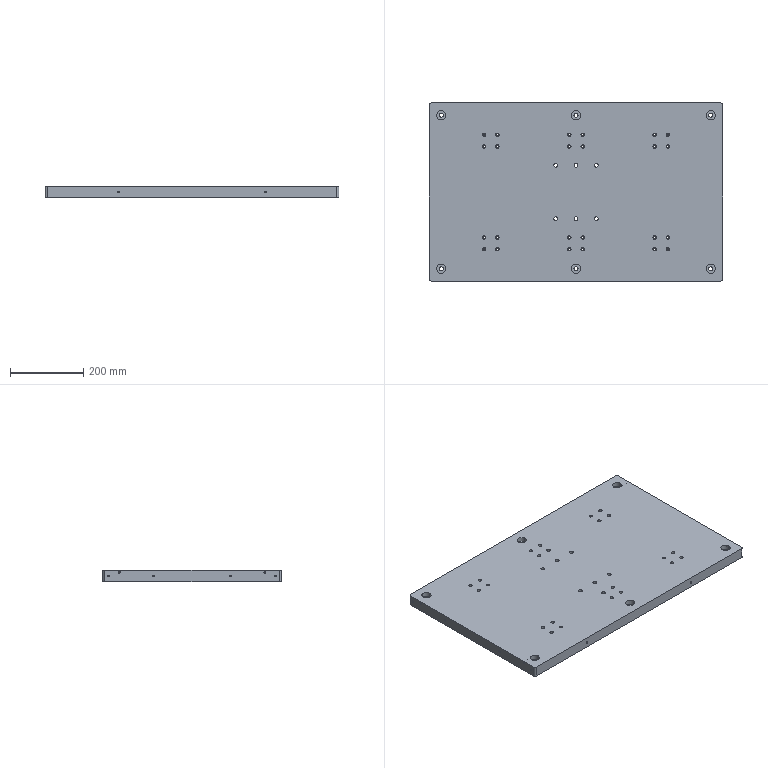NC program | Mastercam | posted with a generic post | part box 800 x 485 x 30 mm
Whole program:
%
O0000()
(MATERIAL - ALUMINUM MM - 2024)
( T20 | 20 FEM | H20 | XY STOCK TO LEAVE - .1 | Z STOCK TO LEAVE - .05 )
( T7 | 4 CHM | H7 )
( T19 | 9 DR | H19 )
( T18 | 8.5 DR | H18 )
( T1 | 10 DR | H1 )
( T14 | 10.5 DR | H14 )
N100 G21
N110 G0 G17 G40 G49 G80 G90
( ?X )
N120 T20 M6
N130 G0 G90 G54 X-410. Y195.1 A0. S5000 M3
N140 G43 H20 Z50. M8
N150 Z1.
N160 G1 Z-.998 F600.
N170 X-390. F4000.
N180 X390.
N190 X410.
N200 Z-1.996 F600.
N210 X390. F4000.
N220 X-390.
N230 X-410.
N240 Z-2.994 F600.
N250 X-390. F4000.
N260 X390.
N270 X410.
N280 Z-3.992 F600.
N290 X390. F4000.
N300 X-390.
N310 X-410.
N320 Z-4.99 F600.
N330 X-390. F4000.
N340 X390.
N350 X410.
N360 Z-5.988 F600.
N370 X390. F4000.
N380 X-390.
N390 X-410.
N400 Z-6.986 F600.
N410 X-390. F4000.
N420 X390.
N430 X410.
N440 Z-7.984 F600.
N450 X390. F4000.
N460 X-390.
N470 X-410.
N480 Z-8.982 F600.
N490 X-390. F4000.
N500 X390.
N510 X410.
N520 Z-9.98 F600.
N530 X390. F4000.
N540 X-390.
N550 X-410.
N560 Z-10.978 F600.
N570 X-390. F4000.
N580 X390.
N590 X410.
N600 Z-11.976 F600.
N610 X390. F4000.
N620 X-390.
N630 X-410.
N640 Z-12.974 F600.
N650 X-390. F4000.
N660 X390.
N670 X410.
N680 Z-13.972 F600.
N690 X390. F4000.
N700 X-390.
N710 X-410.
N720 Z-14.97 F600.
N730 X-390. F4000.
N740 X390.
N750 X410.
N760 Z-15.968 F600.
N770 X390. F4000.
N780 X-390.
N790 X-410.
N800 Z-16.966 F600.
N810 X-390. F4000.
N820 X390.
N830 X410.
N840 Z-17.964 F600.
N850 X390. F4000.
N860 X-390.
N870 X-410.
N880 Z-18.962 F600.
N890 X-390. F4000.
N900 X390.
N910 X410.
N920 Z-19.96 F600.
N930 X390. F4000.
N940 X-390.
N950 X-410.
N960 Z-20.958 F600.
N970 X-390. F4000.
N980 X390.
N990 X410.
N1000 Z-21.956 F600.
N1010 X390. F4000.
N1020 X-390.
N1030 X-410.
N1040 Z-22.954 F600.
N1050 X-390. F4000.
N1060 X390.
N1070 X410.
N1080 Z-23.952 F600.
N1090 X390. F4000.
N1100 X-390.
N1110 X-410.
N1120 Z-24.95 F600.
N1130 X-390. F4000.
N1140 X390.
N1150 X410.
N1160 G0 Z50.
N1170 Y-195.1
N1180 Z1.
N1190 G1 Z-.998 F600.
N1200 X390. F4000.
N1210 X-390.
N1220 X-410.
N1230 Z-1.996 F600.
N1240 X-390. F4000.
N1250 X390.
N1260 X410.
N1270 Z-2.994 F600.
N1280 X390. F4000.
N1290 X-390.
N1300 X-410.
N1310 Z-3.992 F600.
N1320 X-390. F4000.
N1330 X390.
N1340 X410.
N1350 Z-4.99 F600.
N1360 X390. F4000.
N1370 X-390.
N1380 X-410.
N1390 Z-5.988 F600.
N1400 X-390. F4000.
N1410 X390.
N1420 X410.
N1430 Z-6.986 F600.
N1440 X390. F4000.
N1450 X-390.
N1460 X-410.
N1470 Z-7.984 F600.
N1480 X-390. F4000.
N1490 X390.
N1500 X410.
N1510 Z-8.982 F600.
N1520 X390. F4000.
N1530 X-390.
N1540 X-410.
N1550 Z-9.98 F600.
N1560 X-390. F4000.
N1570 X390.
N1580 X410.
N1590 Z-10.978 F600.
N1600 X390. F4000.
N1610 X-390.
N1620 X-410.
N1630 Z-11.976 F600.
N1640 X-390. F4000.
N1650 X390.
N1660 X410.
N1670 Z-12.974 F600.
N1680 X390. F4000.
N1690 X-390.
N1700 X-410.
N1710 Z-13.972 F600.
N1720 X-390. F4000.
N1730 X390.
N1740 X410.
N1750 Z-14.97 F600.
N1760 X390. F4000.
N1770 X-390.
N1780 X-410.
N1790 Z-15.968 F600.
N1800 X-390. F4000.
N1810 X390.
N1820 X410.
N1830 Z-16.966 F600.
N1840 X390. F4000.
N1850 X-390.
N1860 X-410.
N1870 Z-17.964 F600.
N1880 X-390. F4000.
N1890 X390.
N1900 X410.
N1910 Z-18.962 F600.
N1920 X390. F4000.
N1930 X-390.
N1940 X-410.
N1950 Z-19.96 F600.
N1960 X-390. F4000.
N1970 X390.
N1980 X410.
N1990 Z-20.958 F600.
N2000 X390. F4000.
N2010 X-390.
N2020 X-410.
N2030 Z-21.956 F600.
N2040 X-390. F4000.
N2050 X390.
N2060 X410.
N2070 Z-22.954 F600.
N2080 X390. F4000.
N2090 X-390.
N2100 X-410.
N2110 Z-23.952 F600.
N2120 X-390. F4000.
N2130 X390.
N2140 X410.
N2150 Z-24.95 F600.
N2160 X390. F4000.
N2170 X-390.
N2180 X-410.
N2190 G0 Z50.
N2200 Y195.03
N2210 Z1.
N2220 G1 Z-24.95 F600.
N2230 X-390. F1000.
N2240 X390.
N2250 X410.
N2260 G0 Z50.
N2270 X-410. Y195.
N2280 Z1.
N2290 G1 Z-24.95 F600.
N2300 X-390. F1000.
N2310 X390.
N2320 X410.
N2330 G0 Z50.
N2340 Y-195.03
N2350 Z1.
N2360 G1 Z-24.95 F600.
N2370 X390. F1000.
N2380 X-390.
N2390 X-410.
N2400 G0 Z50.
N2410 X410. Y-195.
N2420 Z1.
N2430 G1 Z-24.95 F600.
N2440 X390. F1000.
N2450 X-390.
N2460 X-410.
N2470 G0 Z50.
N2480 M5
N2490 G91 G28 Z0. M9
N2500 A0.
N2510 M01
N2520 T7 M6
N2530 G0 G90 G17 G54 X-394. Y185.65 A0. S6500 M3
N2540 G43 H7 Z50. M8
N2550 Z1.
N2560 G1 Z-.75 F600.
N2570 X-390. F1200.
N2580 X390.
N2590 X394.
N2600 G0 Z50.
N2610 Y-185.65
N2620 Z1.
N2630 G1 Z-.75 F600.
N2640 X390. F1200.
N2650 X-390.
N2660 X-394.
N2670 G0 Z50.
N2680 M5
N2690 G91 G28 Z0. M9
N2700 A0.
N2710 M01
( CCLCY )
M00
N2720 T20 M6
N2730 G0 G90 G17 G54 X388. Y201.1 A0. S5000 M3
N2740 G43 H20 Z50. M8
N2750 Z1.
N2760 G1 Z-.998 F600.
N2770 Y197.1 F4000.
N2780 G3 X390. Y195.1 I2. J0.
N2790 G2 X405.1 Y180. I0. J-15.1
N2800 G1 Y-180.
N2810 G2 X390. Y-195.1 I-15.1 J0.
N2820 G3 X388. Y-197.1 I0. J-2.
N2830 G1 Y-201.1
N2840 Z-1.996 F600.
N2850 Y-197.1 F4000.
N2860 G2 X390. Y-195.1 I2. J0.
N2870 G3 X405.1 Y-180. I0. J15.1
N2880 G1 Y180.
N2890 G3 X390. Y195.1 I-15.1 J0.
N2900 G2 X388. Y197.1 I0. J2.
N2910 G1 Y201.1
N2920 Z-2.994 F600.
N2930 Y197.1 F4000.
N2940 G3 X390. Y195.1 I2. J0.
N2950 G2 X405.1 Y180. I0. J-15.1
N2960 G1 Y-180.
N2970 G2 X390. Y-195.1 I-15.1 J0.
N2980 G3 X388. Y-197.1 I0. J-2.
N2990 G1 Y-201.1
N3000 Z-3.992 F600.
N3010 Y-197.1 F4000.
N3020 G2 X390. Y-195.1 I2. J0.
N3030 G3 X405.1 Y-180. I0. J15.1
N3040 G1 Y180.
N3050 G3 X390. Y195.1 I-15.1 J0.
N3060 G2 X388. Y197.1 I0. J2.
N3070 G1 Y201.1
N3080 Z-4.99 F600.
N3090 Y197.1 F4000.
N3100 G3 X390. Y195.1 I2. J0.
N3110 G2 X405.1 Y180. I0. J-15.1
N3120 G1 Y-180.
N3130 G2 X390. Y-195.1 I-15.1 J0.
N3140 G3 X388. Y-197.1 I0. J-2.
N3150 G1 Y-201.1
N3160 Z-5.988 F600.
N3170 Y-197.1 F4000.
N3180 G2 X390. Y-195.1 I2. J0.
N3190 G3 X405.1 Y-180. I0. J15.1
N3200 G1 Y180.
N3210 G3 X390. Y195.1 I-15.1 J0.
N3220 G2 X388. Y197.1 I0. J2.
N3230 G1 Y201.1
N3240 Z-6.986 F600.
N3250 Y197.1 F4000.
N3260 G3 X390. Y195.1 I2. J0.
N3270 G2 X405.1 Y180. I0. J-15.1
N3280 G1 Y-180.
N3290 G2 X390. Y-195.1 I-15.1 J0.
N3300 G3 X388. Y-197.1 I0. J-2.
N3310 G1 Y-201.1
N3320 Z-7.984 F600.
N3330 Y-197.1 F4000.
N3340 G2 X390. Y-195.1 I2. J0.
N3350 G3 X405.1 Y-180. I0. J15.1
N3360 G1 Y180.
N3370 G3 X390. Y195.1 I-15.1 J0.
N3380 G2 X388. Y197.1 I0. J2.
N3390 G1 Y201.1
N3400 Z-8.982 F600.
N3410 Y197.1 F4000.
N3420 G3 X390. Y195.1 I2. J0.
N3430 G2 X405.1 Y180. I0. J-15.1
N3440 G1 Y-180.
N3450 G2 X390. Y-195.1 I-15.1 J0.
N3460 G3 X388. Y-197.1 I0. J-2.
N3470 G1 Y-201.1
N3480 Z-9.98 F600.
N3490 Y-197.1 F4000.
N3500 G2 X390. Y-195.1 I2. J0.
N3510 G3 X405.1 Y-180. I0. J15.1
N3520 G1 Y180.
N3530 G3 X390. Y195.1 I-15.1 J0.
N3540 G2 X388. Y197.1 I0. J2.
N3550 G1 Y201.1
N3560 Z-10.978 F600.
N3570 Y197.1 F4000.
N3580 G3 X390. Y195.1 I2. J0.
N3590 G2 X405.1 Y180. I0. J-15.1
N3600 G1 Y-180.
N3610 G2 X390. Y-195.1 I-15.1 J0.
N3620 G3 X388. Y-197.1 I0. J-2.
N3630 G1 Y-201.1
N3640 Z-11.976 F600.
N3650 Y-197.1 F4000.
N3660 G2 X390. Y-195.1 I2. J0.
N3670 G3 X405.1 Y-180. I0. J15.1
N3680 G1 Y180.
N3690 G3 X390. Y195.1 I-15.1 J0.
N3700 G2 X388. Y197.1 I0. J2.
N3710 G1 Y201.1
N3720 Z-12.974 F600.
N3730 Y197.1 F4000.
N3740 G3 X390. Y195.1 I2. J0.
N3750 G2 X405.1 Y180. I0. J-15.1
N3760 G1 Y-180.
N3770 G2 X390. Y-195.1 I-15.1 J0.
N3780 G3 X388. Y-197.1 I0. J-2.
N3790 G1 Y-201.1
N3800 Z-13.972 F600.
N3810 Y-197.1 F4000.
N3820 G2 X390. Y-195.1 I2. J0.
N3830 G3 X405.1 Y-180. I0. J15.1
N3840 G1 Y180.
N3850 G3 X390. Y195.1 I-15.1 J0.
N3860 G2 X388. Y197.1 I0. J2.
N3870 G1 Y201.1
N3880 Z-14.97 F600.
N3890 Y197.1 F4000.
N3900 G3 X390. Y195.1 I2. J0.
N3910 G2 X405.1 Y180. I0. J-15.1
N3920 G1 Y-180.
N3930 G2 X390. Y-195.1 I-15.1 J0.
N3940 G3 X388. Y-197.1 I0. J-2.
N3950 G1 Y-201.1
N3960 Z-15.968 F600.
N3970 Y-197.1 F4000.
N3980 G2 X390. Y-195.1 I2. J0.
N3990 G3 X405.1 Y-180. I0. J15.1
N4000 G1 Y180.
N4010 G3 X390. Y195.1 I-15.1 J0.
N4020 G2 X388. Y197.1 I0. J2.
N4030 G1 Y201.1
N4040 Z-16.966 F600.
N4050 Y197.1 F4000.
N4060 G3 X390. Y195.1 I2. J0.
N4070 G2 X405.1 Y180. I0. J-15.1
N4080 G1 Y-180.
N4090 G2 X390. Y-195.1 I-15.1 J0.
N4100 G3 X388. Y-197.1 I0. J-2.
N4110 G1 Y-201.1
N4120 Z-17.964 F600.
N4130 Y-197.1 F4000.
N4140 G2 X390. Y-195.1 I2. J0.
N4150 G3 X405.1 Y-180. I0. J15.1
N4160 G1 Y180.
N4170 G3 X390. Y195.1 I-15.1 J0.
N4180 G2 X388. Y197.1 I0. J2.
N4190 G1 Y201.1
N4200 Z-18.962 F600.
N4210 Y197.1 F4000.
N4220 G3 X390. Y195.1 I2. J0.
N4230 G2 X405.1 Y180. I0. J-15.1
N4240 G1 Y-180.
N4250 G2 X390. Y-195.1 I-15.1 J0.
N4260 G3 X388. Y-197.1 I0. J-2.
N4270 G1 Y-201.1
N4280 Z-19.96 F600.
N4290 Y-197.1 F4000.
N4300 G2 X390. Y-195.1 I2. J0.
N4310 G3 X405.1 Y-180. I0. J15.1
N4320 G1 Y180.
N4330 G3 X390. Y195.1 I-15.1 J0.
N4340 G2 X388. Y197.1 I0. J2.
N4350 G1 Y201.1
N4360 Z-20.958 F600.
N4370 Y197.1 F4000.
N4380 G3 X390. Y195.1 I2. J0.
N4390 G2 X405.1 Y180. I0. J-15.1
N4400 G1 Y-180.
N4410 G2 X390. Y-195.1 I-15.1 J0.
N4420 G3 X388. Y-197.1 I0. J-2.
N4430 G1 Y-201.1
N4440 Z-21.956 F600.
N4450 Y-197.1 F4000.
N4460 G2 X390. Y-195.1 I2. J0.
N4470 G3 X405.1 Y-180. I0. J15.1
N4480 G1 Y180.
N4490 G3 X390. Y195.1 I-15.1 J0.
N4500 G2 X388. Y197.1 I0. J2.
N4510 G1 Y201.1
N4520 Z-22.954 F600.
N4530 Y197.1 F4000.
N4540 G3 X390. Y195.1 I2. J0.
N4550 G2 X405.1 Y180. I0. J-15.1
N4560 G1 Y-180.
N4570 G2 X390. Y-195.1 I-15.1 J0.
N4580 G3 X388. Y-197.1 I0. J-2.
N4590 G1 Y-201.1
N4600 Z-23.952 F600.
N4610 Y-197.1 F4000.
N4620 G2 X390. Y-195.1 I2. J0.
N4630 G3 X405.1 Y-180. I0. J15.1
N4640 G1 Y180.
N4650 G3 X390. Y195.1 I-15.1 J0.
N4660 G2 X388. Y197.1 I0. J2.
N4670 G1 Y201.1
N4680 Z-24.95 F600.
N4690 Y197.1 F4000.
N4700 G3 X390. Y195.1 I2. J0.
N4710 G2 X405.1 Y180. I0. J-15.1
N4720 G1 Y-180.
N4730 G2 X390. Y-195.1 I-15.1 J0.
N4740 G3 X388. Y-197.1 I0. J-2.
N4750 G1 Y-201.1
N4760 G0 Z50.
N4770 X-388.
N4780 Z1.
N4790 G1 Z-.998 F600.
N4800 Y-197.1 F4000.
N4810 G3 X-390. Y-195.1 I-2. J0.
N4820 G2 X-405.1 Y-180. I0. J15.1
N4830 G1 Y180.
N4840 G2 X-390. Y195.1 I15.1 J0.
N4850 G3 X-388. Y197.1 I0. J2.
N4860 G1 Y201.1
N4870 Z-1.996 F600.
N4880 Y197.1 F4000.
N4890 G2 X-390. Y195.1 I-2. J0.
N4900 G3 X-405.1 Y180. I0. J-15.1
N4910 G1 Y-180.
N4920 G3 X-390. Y-195.1 I15.1 J0.
N4930 G2 X-388. Y-197.1 I0. J-2.
N4940 G1 Y-201.1
N4950 Z-2.994 F600.
N4960 Y-197.1 F4000.
N4970 G3 X-390. Y-195.1 I-2. J0.
N4980 G2 X-405.1 Y-180. I0. J15.1
N4990 G1 Y180.
N5000 G2 X-390. Y195.1 I15.1 J0.
N5010 G3 X-388. Y197.1 I0. J2.
N5020 G1 Y201.1
N5030 Z-3.992 F600.
N5040 Y197.1 F4000.
N5050 G2 X-390. Y195.1 I-2. J0.
N5060 G3 X-405.1 Y180. I0. J-15.1
N5070 G1 Y-180.
N5080 G3 X-390. Y-195.1 I15.1 J0.
N5090 G2 X-388. Y-197.1 I0. J-2.
N5100 G1 Y-201.1
N5110 Z-4.99 F600.
N5120 Y-197.1 F4000.
N5130 G3 X-390. Y-195.1 I-2. J0.
N5140 G2 X-405.1 Y-180. I0. J15.1
N5150 G1 Y180.
N5160 G2 X-390. Y195.1 I15.1 J0.
N5170 G3 X-388. Y197.1 I0. J2.
N5180 G1 Y201.1
N5190 Z-5.988 F600.
N5200 Y197.1 F4000.
N5210 G2 X-390. Y195.1 I-2. J0.
N5220 G3 X-405.1 Y180. I0. J-15.1
N5230 G1 Y-180.
N5240 G3 X-390. Y-195.1 I15.1 J0.
N5250 G2 X-388. Y-197.1 I0. J-2.
N5260 G1 Y-201.1
N5270 Z-6.986 F600.
N5280 Y-197.1 F4000.
N5290 G3 X-390. Y-195.1 I-2. J0.
N5300 G2 X-405.1 Y-180. I0. J15.1
N5310 G1 Y180.
N5320 G2 X-390. Y195.1 I15.1 J0.
N5330 G3 X-388. Y197.1 I0. J2.
N5340 G1 Y201.1
N5350 Z-7.984 F600.
N5360 Y197.1 F4000.
N5370 G2 X-390. Y195.1 I-2. J0.
N5380 G3 X-405.1 Y180. I0. J-15.1
N5390 G1 Y-180.
N5400 G3 X-390. Y-195.1 I15.1 J0.
N5410 G2 X-388. Y-197.1 I0. J-2.
N5420 G1 Y-201.1
N5430 Z-8.982 F600.
N5440 Y-197.1 F4000.
N5450 G3 X-390. Y-195.1 I-2. J0.
N5460 G2 X-405.1 Y-180. I0. J15.1
N5470 G1 Y180.
N5480 G2 X-390. Y195.1 I15.1 J0.
N5490 G3 X-388. Y197.1 I0. J2.
N5500 G1 Y201.1
N5510 Z-9.98 F600.
N5520 Y197.1 F4000.
N5530 G2 X-390. Y195.1 I-2. J0.
N5540 G3 X-405.1 Y180. I0. J-15.1
N5550 G1 Y-180.
N5560 G3 X-390. Y-195.1 I15.1 J0.
N5570 G2 X-388. Y-197.1 I0. J-2.
N5580 G1 Y-201.1
N5590 Z-10.978 F600.
N5600 Y-197.1 F4000.
N5610 G3 X-390. Y-195.1 I-2. J0.
N5620 G2 X-405.1 Y-180. I0. J15.1
N5630 G1 Y180.
N5640 G2 X-390. Y195.1 I15.1 J0.
N5650 G3 X-388. Y197.1 I0. J2.
N5660 G1 Y201.1
N5670 Z-11.976 F600.
N5680 Y197.1 F4000.
N5690 G2 X-390. Y195.1 I-2. J0.
N5700 G3 X-405.1 Y180. I0. J-15.1
N5710 G1 Y-180.
N5720 G3 X-390. Y-195.1 I15.1 J0.
N5730 G2 X-388. Y-197.1 I0. J-2.
N5740 G1 Y-201.1
N5750 Z-12.974 F600.
N5760 Y-197.1 F4000.
N5770 G3 X-390. Y-195.1 I-2. J0.
N5780 G2 X-405.1 Y-180. I0. J15.1
N5790 G1 Y180.
N5800 G2 X-390. Y195.1 I15.1 J0.
N5810 G3 X-388. Y197.1 I0. J2.
N5820 G1 Y201.1
N5830 Z-13.972 F600.
N5840 Y197.1 F4000.
N5850 G2 X-390. Y195.1 I-2. J0.
N5860 G3 X-405.1 Y180. I0. J-15.1
N5870 G1 Y-180.
N5880 G3 X-390. Y-195.1 I15.1 J0.
N5890 G2 X-388. Y-197.1 I0. J-2.
N5900 G1 Y-201.1
N5910 Z-14.97 F600.
N5920 Y-197.1 F4000.
N5930 G3 X-390. Y-195.1 I-2. J0.
N5940 G2 X-405.1 Y-180. I0. J15.1
N5950 G1 Y180.
N5960 G2 X-390. Y195.1 I15.1 J0.
N5970 G3 X-388. Y197.1 I0. J2.
N5980 G1 Y201.1
N5990 Z-15.968 F600.
N6000 Y197.1 F4000.
N6010 G2 X-390. Y195.1 I-2. J0.
N6020 G3 X-405.1 Y180. I0. J-15.1
N6030 G1 Y-180.
N6040 G3 X-390. Y-195.1 I15.1 J0.
N6050 G2 X-388. Y-197.1 I0. J-2.
N6060 G1 Y-201.1
N6070 Z-16.966 F600.
N6080 Y-197.1 F4000.
N6090 G3 X-390. Y-195.1 I-2. J0.
N6100 G2 X-405.1 Y-180. I0. J15.1
N6110 G1 Y180.
N6120 G2 X-390. Y195.1 I15.1 J0.
N6130 G3 X-388. Y197.1 I0. J2.
N6140 G1 Y201.1
N6150 Z-17.964 F600.
N6160 Y197.1 F4000.
N6170 G2 X-390. Y195.1 I-2. J0.
N6180 G3 X-405.1 Y180. I0. J-15.1
N6190 G1 Y-180.
N6200 G3 X-390. Y-195.1 I15.1 J0.
N6210 G2 X-388. Y-197.1 I0. J-2.
N6220 G1 Y-201.1
N6230 Z-18.962 F600.
N6240 Y-197.1 F4000.
N6250 G3 X-390. Y-195.1 I-2. J0.
N6260 G2 X-405.1 Y-180. I0. J15.1
N6270 G1 Y180.
N6280 G2 X-390. Y195.1 I15.1 J0.
N6290 G3 X-388. Y197.1 I0. J2.
N6300 G1 Y201.1
N6310 Z-19.96 F600.
N6320 Y197.1 F4000.
N6330 G2 X-390. Y195.1 I-2. J0.
N6340 G3 X-405.1 Y180. I0. J-15.1
N6350 G1 Y-180.
N6360 G3 X-390. Y-195.1 I15.1 J0.
N6370 G2 X-388. Y-197.1 I0. J-2.
N6380 G1 Y-201.1
N6390 Z-20.958 F600.
N6400 Y-197.1 F4000.
N6410 G3 X-390. Y-195.1 I-2. J0.
N6420 G2 X-405.1 Y-180. I0. J15.1
N6430 G1 Y180.
N6440 G2 X-390. Y195.1 I15.1 J0.
N6450 G3 X-388. Y197.1 I0. J2.
N6460 G1 Y201.1
N6470 Z-21.956 F600.
N6480 Y197.1 F4000.
N6490 G2 X-390. Y195.1 I-2. J0.
N6500 G3 X-405.1 Y180. I0. J-15.1
N6510 G1 Y-180.
N6520 G3 X-390. Y-195.1 I15.1 J0.
N6530 G2 X-388. Y-197.1 I0. J-2.
N6540 G1 Y-201.1
N6550 Z-22.954 F600.
N6560 Y-197.1 F4000.
N6570 G3 X-390. Y-195.1 I-2. J0.
N6580 G2 X-405.1 Y-180. I0. J15.1
N6590 G1 Y180.
N6600 G2 X-390. Y195.1 I15.1 J0.
N6610 G3 X-388. Y197.1 I0. J2.
N6620 G1 Y201.1
N6630 Z-23.952 F600.
N6640 Y197.1 F4000.
N6650 G2 X-390. Y195.1 I-2. J0.
N6660 G3 X-405.1 Y180. I0. J-15.1
N6670 G1 Y-180.
N6680 G3 X-390. Y-195.1 I15.1 J0.
N6690 G2 X-388. Y-197.1 I0. J-2.
N6700 G1 Y-201.1
N6710 Z-24.95 F600.
N6720 Y-197.1 F4000.
N6730 G3 X-390. Y-195.1 I-2. J0.
N6740 G2 X-405.1 Y-180. I0. J15.1
N6750 G1 Y180.
N6760 G2 X-390. Y195.1 I15.1 J0.
N6770 G3 X-388. Y197.1 I0. J2.
N6780 G1 Y201.1
N6790 G0 Z50.
N6800 X388. Y201.03
N6810 Z1.
N6820 G1 Z-24.95 F600.
N6830 Y197.03 F1000.
N6840 G3 X390. Y195.03 I2. J0.
N6850 G2 X405.03 Y180. I0. J-15.03
N6860 G1 Y-180.
N6870 G2 X390. Y-195.03 I-15.03 J0.
N6880 G3 X388. Y-197.03 I0. J-2.
N6890 G1 Y-201.03
N6900 G0 Z50.
N6910 Y201.
N6920 Z1.
N6930 G1 Z-24.95 F600.
N6940 Y197. F1000.
N6950 G3 X390. Y195. I2. J0.
N6960 G2 X405. Y180. I0. J-15.
N6970 G1 Y-180.
N6980 G2 X390. Y-195. I-15. J0.
N6990 G3 X388. Y-197. I0. J-2.
N7000 G1 Y-201.
N7010 G0 Z50.
N7020 X-388. Y-201.03
N7030 Z1.
N7040 G1 Z-24.95 F600.
N7050 Y-197.03 F1000.
N7060 G3 X-390. Y-195.03 I-2. J0.
N7070 G2 X-405.03 Y-180. I0. J15.03
N7080 G1 Y180.
N7090 G2 X-390. Y195.03 I15.03 J0.
N7100 G3 X-388. Y197.03 I0. J2.
N7110 G1 Y201.03
N7120 G0 Z50.
N7130 Y-201.
N7140 Z1.
N7150 G1 Z-24.95 F600.
N7160 Y-197. F1000.
N7170 G3 X-390. Y-195. I-2. J0.
N7180 G2 X-405. Y-180. I0. J15.
N7190 G1 Y180.
N7200 G2 X-390. Y195. I15. J0.
N7210 G3 X-388. Y197. I0. J2.
N7220 G1 Y201.
N7230 G0 Z50.
N7240 M5
N7250 G91 G28 Z0. M9
N7260 A0.
N7270 M01
N7280 T7 M6
N7290 G0 G90 G17 G54 X389.6 Y186.85 A0. S6500 M3
N7300 G43 H7 Z50. M8
N7310 Z1.
N7320 G1 Z-.75 F600.
N7330 Y186.05 F1000.
N7340 G3 X390. Y185.65 I.4 J0.
N7350 G2 X395.65 Y180. I0. J-5.65
N7360 G1 Y-180.
N7370 G2 X390. Y-185.65 I-5.65 J0.
N7380 G3 X389.6 Y-186.05 I0. J-.4
N7390 G1 Y-186.85
N7400 G0 Z50.
N7410 X-389.6
N7420 Z1.
N7430 G1 Z-.75 F600.
N7440 Y-186.05 F1000.
N7450 G3 X-390. Y-185.65 I-.4 J0.
N7460 G2 X-395.65 Y-180. I0. J5.65
N7470 G1 Y180.
N7480 G2 X-390. Y185.65 I5.65 J0.
N7490 G3 X-389.6 Y186.05 I0. J.4
N7500 G1 Y186.85
N7510 G0 Z50.
N7520 S6000 M3
N7530 M9
N7540 X300. Y-160.
N7550 G98 G81 Z-.7 R1. F200.
N7560 X365. Y-120.
N7570 X265. Y0.
N7580 X365. Y120.
N7590 X300. Y160.
N7600 X150.
N7610 X100.
N7620 X0.
N7630 X-100.
N7640 X-150.
N7650 X-300.
N7660 X-365. Y120.
N7670 X-265. Y0.
N7680 X-365. Y-120.
N7690 X-300. Y-160.
N7700 X-150.
N7710 X-100.
N7720 X0.
N7730 X100.
N7740 X150.
N7750 G80
N7760 M5
N7770 G91 G0 G28 Z0.
N7780 A0.
N7790 M01
N7800 T19 M6
N7810 G0 G90 G17 G54 X300. Y-160. A0. S800 M3
N7820 G43 H19 Z50.
N7830 G98 G83 Z-24.8 R1. Q2. F100.
N7840 X100.
N7850 X-100.
N7860 X-300.
N7870 Y160.
N7880 X-100.
N7890 X100.
N7900 X300.
N7910 G80
N7920 M5
N7930 G91 G0 G28 Z0.
N7940 A0.
N7950 M01
N7960 T18 M6
N7970 G0 G90 G17 G54 X365. Y-120. A0. S800 M3
N7980 G43 H18 Z50.
N7990 G98 G83 Z-24.8 R1. Q2. F100.
N8000 X265. Y0.
N8010 X365. Y120.
N8020 X150. Y160.
N8030 X0.
N8040 X-150.
N8050 X-365. Y120.
N8060 X-265. Y0.
N8070 X-365. Y-120.
N8080 X-150. Y-160.
N8090 X0.
N8100 X150.
N8110 G80
N8120 M5
N8130 G91 G0 G28 Z0.
N8140 A0.
N8150 M01
N8160 T7 M6
N8170 G0 G90 G17 G54 X-297.35 Y159.6 A0. S6500 M3
N8180 G43 H7 Z50. M8
N8190 Z1.
N8200 G1 Z-.8 F600.
N8210 X-296.55 F1200.
N8220 G3 X-296.15 Y160. I0. J.4
N8230 X-300. Y163.85 I-3.85 J0.
N8240 X-303.85 Y160. I0. J-3.85
N8250 X-300. Y156.15 I3.85 J0.
N8260 X-296.15 Y160. I0. J3.85
N8270 X-296.55 Y160.4 I-.4 J0.
N8280 G1 X-297.35
N8290 G0 Z50.
N8300 X-262.5 Y-.4
N8310 Z1.
N8320 G1 Z-.8 F600.
N8330 X-261.7 F1200.
N8340 G3 X-261.3 Y0. I0. J.4
N8350 X-265. Y3.7 I-3.7 J0.
N8360 X-268.7 Y0. I0. J-3.7
N8370 X-265. Y-3.7 I3.7 J0.
N8380 X-261.3 Y0. I0. J3.7
N8390 X-261.7 Y.4 I-.4 J0.
N8400 G1 X-262.5
N8410 G0 Z50.
N8420 X-362.5 Y-120.4
N8430 Z1.
N8440 G1 Z-.8 F600.
N8450 X-361.7 F1200.
N8460 G3 X-361.3 Y-120. I0. J.4
N8470 X-365. Y-116.3 I-3.7 J0.
N8480 X-368.7 Y-120. I0. J-3.7
N8490 X-365. Y-123.7 I3.7 J0.
N8500 X-361.3 Y-120. I0. J3.7
N8510 X-361.7 Y-119.6 I-.4 J0.
N8520 G1 X-362.5
N8530 G0 Z50.
N8540 X-297.35 Y-160.4
N8550 Z1.
N8560 G1 Z-.8 F600.
N8570 X-296.55 F1200.
N8580 G3 X-296.15 Y-160. I0. J.4
N8590 X-300. Y-156.15 I-3.85 J0.
N8600 X-303.85 Y-160. I0. J-3.85
N8610 X-300. Y-163.85 I3.85 J0.
N8620 X-296.15 Y-160. I0. J3.85
N8630 X-296.55 Y-159.6 I-.4 J0.
N8640 G1 X-297.35
N8650 G0 Z50.
N8660 X-147.5 Y-160.4
N8670 Z1.
N8680 G1 Z-.8 F600.
N8690 X-146.7 F1200.
N8700 G3 X-146.3 Y-160. I0. J.4
N8710 X-150. Y-156.3 I-3.7 J0.
N8720 X-153.7 Y-160. I0. J-3.7
N8730 X-150. Y-163.7 I3.7 J0.
N8740 X-146.3 Y-160. I0. J3.7
N8750 X-146.7 Y-159.6 I-.4 J0.
N8760 G1 X-147.5
N8770 G0 Z50.
N8780 X-97.35 Y-160.4
N8790 Z1.
N8800 G1 Z-.8 F600.
N8810 X-96.55 F1200.
N8820 G3 X-96.15 Y-160. I0. J.4
N8830 X-100. Y-156.15 I-3.85 J0.
N8840 X-103.85 Y-160. I0. J-3.85
N8850 X-100. Y-163.85 I3.85 J0.
N8860 X-96.15 Y-160. I0. J3.85
N8870 X-96.55 Y-159.6 I-.4 J0.
N8880 G1 X-97.35
N8890 G0 Z50.
N8900 X-147.5 Y159.6
N8910 Z1.
N8920 G1 Z-.8 F600.
N8930 X-146.7 F1200.
N8940 G3 X-146.3 Y160. I0. J.4
N8950 X-150. Y163.7 I-3.7 J0.
N8960 X-153.7 Y160. I0. J-3.7
N8970 X-150. Y156.3 I3.7 J0.
N8980 X-146.3 Y160. I0. J3.7
N8990 X-146.7 Y160.4 I-.4 J0.
N9000 G1 X-147.5
N9010 G0 Z50.
N9020 X-97.35 Y159.6
N9030 Z1.
N9040 G1 Z-.8 F600.
N9050 X-96.55 F1200.
N9060 G3 X-96.15 Y160. I0. J.4
N9070 X-100. Y163.85 I-3.85 J0.
N9080 X-103.85 Y160. I0. J-3.85
N9090 X-100. Y156.15 I3.85 J0.
N9100 X-96.15 Y160. I0. J3.85
N9110 X-96.55 Y160.4 I-.4 J0.
N9120 G1 X-97.35
N9130 G0 Z50.
N9140 X2.5 Y159.6
N9150 Z1.
N9160 G1 Z-.8 F600.
N9170 X3.3 F1200.
N9180 G3 X3.7 Y160. I0. J.4
N9190 X0. Y163.7 I-3.7 J0.
N9200 X-3.7 Y160. I0. J-3.7
N9210 X0. Y156.3 I3.7 J0.
N9220 X3.7 Y160. I0. J3.7
N9230 X3.3 Y160.4 I-.4 J0.
N9240 G1 X2.5
N9250 G0 Z50.
N9260 X102.65 Y159.6
N9270 Z1.
N9280 G1 Z-.8 F600.
N9290 X103.45 F1200.
N9300 G3 X103.85 Y160. I0. J.4
N9310 X100. Y163.85 I-3.85 J0.
N9320 X96.15 Y160. I0. J-3.85
N9330 X100. Y156.15 I3.85 J0.
N9340 X103.85 Y160. I0. J3.85
N9350 X103.45 Y160.4 I-.4 J0.
N9360 G1 X102.65
N9370 G0 Z50.
N9380 X152.5 Y159.6
N9390 Z1.
N9400 G1 Z-.8 F600.
N9410 X153.3 F1200.
N9420 G3 X153.7 Y160. I0. J.4
N9430 X150. Y163.7 I-3.7 J0.
N9440 X146.3 Y160. I0. J-3.7
N9450 X150. Y156.3 I3.7 J0.
N9460 X153.7 Y160. I0. J3.7
N9470 X153.3 Y160.4 I-.4 J0.
N9480 G1 X152.5
N9490 G0 Z50.
N9500 X302.65 Y159.6
N9510 Z1.
N9520 G1 Z-.8 F600.
N9530 X303.45 F1200.
N9540 G3 X303.85 Y160. I0. J.4
N9550 X300. Y163.85 I-3.85 J0.
N9560 X296.15 Y160. I0. J-3.85
N9570 X300. Y156.15 I3.85 J0.
N9580 X303.85 Y160. I0. J3.85
N9590 X303.45 Y160.4 I-.4 J0.
N9600 G1 X302.65
N9610 G0 Z50.
N9620 X367.5 Y119.6
N9630 Z1.
N9640 G1 Z-.8 F600.
N9650 X368.3 F1200.
N9660 G3 X368.7 Y120. I0. J.4
N9670 X365. Y123.7 I-3.7 J0.
N9680 X361.3 Y120. I0. J-3.7
N9690 X365. Y116.3 I3.7 J0.
N9700 X368.7 Y120. I0. J3.7
N9710 X368.3 Y120.4 I-.4 J0.
N9720 G1 X367.5
N9730 G0 Z50.
N9740 X267.5 Y-.4
N9750 Z1.
N9760 G1 Z-.8 F600.
N9770 X268.3 F1200.
N9780 G3 X268.7 Y0. I0. J.4
N9790 X265. Y3.7 I-3.7 J0.
N9800 X261.3 Y0. I0. J-3.7
N9810 X265. Y-3.7 I3.7 J0.
N9820 X268.7 Y0. I0. J3.7
N9830 X268.3 Y.4 I-.4 J0.
N9840 G1 X267.5
N9850 G0 Z50.
N9860 X367.5 Y-120.4
N9870 Z1.
N9880 G1 Z-.8 F600.
N9890 X368.3 F1200.
N9900 G3 X368.7 Y-120. I0. J.4
N9910 X365. Y-116.3 I-3.7 J0.
N9920 X361.3 Y-120. I0. J-3.7
N9930 X365. Y-123.7 I3.7 J0.
N9940 X368.7 Y-120. I0. J3.7
N9950 X368.3 Y-119.6 I-.4 J0.
N9960 G1 X367.5
N9970 G0 Z50.
N9980 X302.65 Y-160.4
N9990 Z1.
N100 G1 Z-.8 F600.
N110 X303.45 F1200.
N120 G3 X303.85 Y-160. I0. J.4
N130 X300. Y-156.15 I-3.85 J0.
N140 X296.15 Y-160. I0. J-3.85
N150 X300. Y-163.85 I3.85 J0.
N160 X303.85 Y-160. I0. J3.85
N170 X303.45 Y-159.6 I-.4 J0.
N180 G1 X302.65
N190 G0 Z50.
N200 X152.5 Y-160.4
N210 Z1.
N220 G1 Z-.8 F600.
N230 X153.3 F1200.
N240 G3 X153.7 Y-160. I0. J.4
N250 X150. Y-156.3 I-3.7 J0.
N260 X146.3 Y-160. I0. J-3.7
N270 X150. Y-163.7 I3.7 J0.
N280 X153.7 Y-160. I0. J3.7
N290 X153.3 Y-159.6 I-.4 J0.
N300 G1 X152.5
N310 G0 Z50.
N320 X102.65 Y-160.4
N330 Z1.
N340 G1 Z-.8 F600.
N350 X103.45 F1200.
N360 G3 X103.85 Y-160. I0. J.4
N370 X100. Y-156.15 I-3.85 J0.
N380 X96.15 Y-160. I0. J-3.85
N390 X100. Y-163.85 I3.85 J0.
N400 X103.85 Y-160. I0. J3.85
N410 X103.45 Y-159.6 I-.4 J0.
N420 G1 X102.65
N430 G0 Z50.
N440 X2.5 Y-160.4
N450 Z1.
N460 G1 Z-.8 F600.
N470 X3.3 F1200.
N480 G3 X3.7 Y-160. I0. J.4
N490 X0. Y-156.3 I-3.7 J0.
N500 X-3.7 Y-160. I0. J-3.7
N510 X0. Y-163.7 I3.7 J0.
N520 X3.7 Y-160. I0. J3.7
N530 X3.3 Y-159.6 I-.4 J0.
N540 G1 X2.5
N550 G0 Z50.
N560 X-362.5 Y119.6
N570 Z1.
N580 G1 Z-.8 F600.
N590 X-361.7 F1200.
N600 G3 X-361.3 Y120. I0. J.4
N610 X-365. Y123.7 I-3.7 J0.
N620 X-368.7 Y120. I0. J-3.7
N630 X-365. Y116.3 I3.7 J0.
N640 X-361.3 Y120. I0. J3.7
N650 X-361.7 Y120.4 I-.4 J0.
N660 G1 X-362.5
N670 G0 Z50.
N680 S6000 M3
N690 M9
N700 X330. Y0.
N710 G98 G81 Z-.7 R1. F200.
N720 X265.
N730 X198.
N740 X66.
N750 X-66.
N760 X-198.
N770 X-265.
N780 X-330.
N790 G80
N800 M5
N810 G91 G0 G28 Z0.
N820 A0.
N830 M01
N840 T1 M6
N850 G0 G90 G17 G54 X330. Y0. A0. S800 M3
N860 G43 H1 Z50.
N870 G98 G83 Z-50. R1. Q2. F80.
N880 X198.
N890 X66.
N900 X-66.
N910 X-198.
N920 X-330.
N930 G80
N940 M5
N950 G91 G0 G28 Z0.
N960 A0.
N970 M01
N980 T14 M6
N990 G0 G90 G17 G54 X-265. Y0. A0. S800 M3
N1000 G43 H14 Z50.
N1010 G98 G83 Z-25. R1. Q2. F80.
N1020 X265.
N1030 G80
N1040 M5
N1050 G91 G0 G28 Z0.
N1060 A0.
N1070 M01
N1080 T7 M6
N1090 G0 G90 G17 G54 X-261.6 Y-.4 A0. S6500 M3
N1100 G43 H7 Z50. M8
N1110 Z1.
N1120 G1 Z-.8 F600.
N1130 X-260.8 F1200.
N1140 G3 X-260.4 Y0. I0. J.4
N1150 X-265. Y4.6 I-4.6 J0.
N1160 X-269.6 Y0. I0. J-4.6
N1170 X-265. Y-4.6 I4.6 J0.
N1180 X-260.4 Y0. I0. J4.6
N1190 X-260.8 Y.4 I-.4 J0.
N1200 G1 X-261.6
N1210 G0 Z50.
N1220 X268.4 Y-.4
N1230 Z1.
N1240 G1 Z-.8 F600.
N1250 X269.2 F1200.
N1260 G3 X269.6 Y0. I0. J.4
N1270 X265. Y4.6 I-4.6 J0.
N1280 X260.4 Y0. I0. J-4.6
N1290 X265. Y-4.6 I4.6 J0.
N1300 X269.6 Y0. I0. J4.6
N1310 X269.2 Y.4 I-.4 J0.
N1320 G1 X268.4
N1330 G0 Z50.
N1340 X-194.85 Y-.4
N1350 Z1.
N1360 G1 Z-.8 F600.
N1370 X-194.05 F1200.
N1380 G3 X-193.65 Y0. I0. J.4
N1390 X-198. Y4.35 I-4.35 J0.
N1400 X-202.35 Y0. I0. J-4.35
N1410 X-198. Y-4.35 I4.35 J0.
N1420 X-193.65 Y0. I0. J4.35
N1430 X-194.05 Y.4 I-.4 J0.
N1440 G1 X-194.85
N1450 G0 Z50.
N1460 X-62.85 Y-.4
N1470 Z1.
N1480 G1 Z-.8 F600.
N1490 X-62.05 F1200.
N1500 G3 X-61.65 Y0. I0. J.4
N1510 X-66. Y4.35 I-4.35 J0.
N1520 X-70.35 Y0. I0. J-4.35
N1530 X-66. Y-4.35 I4.35 J0.
N1540 X-61.65 Y0. I0. J4.35
N1550 X-62.05 Y.4 I-.4 J0.
N1560 G1 X-62.85
N1570 G0 Z50.
N1580 X69.15 Y-.4
N1590 Z1.
N1600 G1 Z-.8 F600.
N1610 X69.95 F1200.
N1620 G3 X70.35 Y0. I0. J.4
N1630 X66. Y4.35 I-4.35 J0.
N1640 X61.65 Y0. I0. J-4.35
N1650 X66. Y-4.35 I4.35 J0.
N1660 X70.35 Y0. I0. J4.35
N1670 X69.95 Y.4 I-.4 J0.
N1680 G1 X69.15
N1690 G0 Z50.
N1700 X201.15 Y-.4
N1710 Z1.
N1720 G1 Z-.8 F600.
N1730 X201.95 F1200.
N1740 G3 X202.35 Y0. I0. J.4
N1750 X198. Y4.35 I-4.35 J0.
N1760 X193.65 Y0. I0. J-4.35
N1770 X198. Y-4.35 I4.35 J0.
N1780 X202.35 Y0. I0. J4.35
N1790 X201.95 Y.4 I-.4 J0.
N1800 G1 X201.15
N1810 G0 Z50.
N1820 X333.15 Y-.4
N1830 Z1.
N1840 G1 Z-.8 F600.
N1850 X333.95 F1200.
N1860 G3 X334.35 Y0. I0. J.4
N1870 X330. Y4.35 I-4.35 J0.
N1880 X325.65 Y0. I0. J-4.35
N1890 X330. Y-4.35 I4.35 J0.
N1900 X334.35 Y0. I0. J4.35
N1910 X333.95 Y.4 I-.4 J0.
N1920 G1 X333.15
N1930 G0 Z50.
N1940 X-326.85 Y-.4
N1950 Z1.
N1960 G1 Z-.8 F600.
N1970 X-326.05 F1200.
N1980 G3 X-325.65 Y0. I0. J.4
N1990 X-330. Y4.35 I-4.35 J0.
N2000 X-334.35 Y0. I0. J-4.35
N2010 X-330. Y-4.35 I4.35 J0.
N2020 X-325.65 Y0. I0. J4.35
N2030 X-326.05 Y.4 I-.4 J0.
N2040 G1 X-326.85
N2050 G0 Z50.
N2060 M5
N2070 G91 G28 Z0. M9
N2080 G28 X0. Y0. A0.
N2090 M30
%